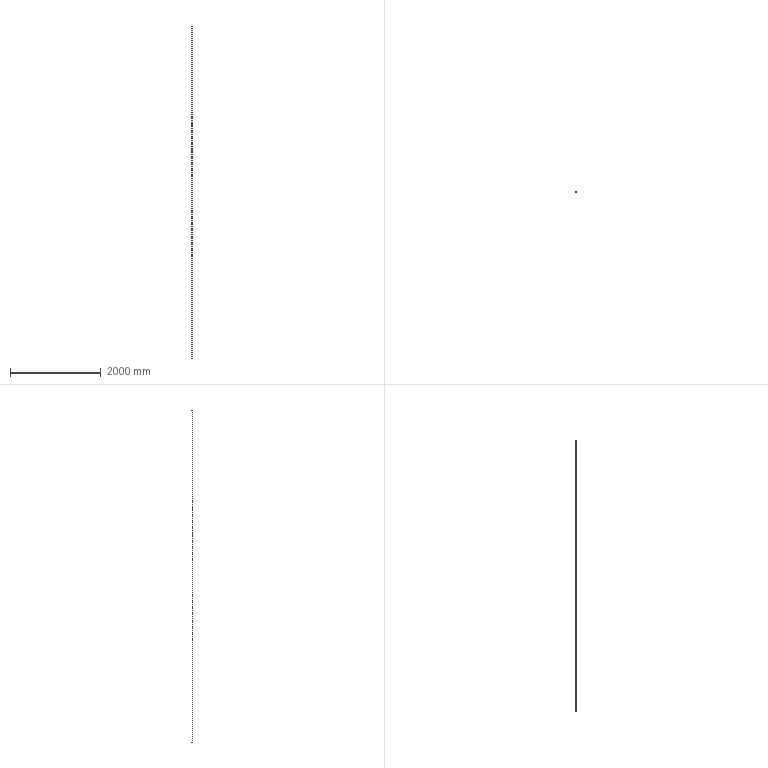Part | SolidWorks | features Extrusion 1 | 1 solid | 6 faces | box 19.05 x 19.05 x 7329 mm | volume 1032084 mm3 | cylinder 4 | plane 2 | commonest cylinder face diameters 13.55 x2 19.05 x2
STEP:
#1=CARTESIAN_POINT('',(-6.775,0.,3664.5));
#2=VERTEX_POINT('',#1);
#3=CARTESIAN_POINT('',(6.775,0.,3664.5));
#4=VERTEX_POINT('',#3);
#5=CARTESIAN_POINT('',(0.,0.,3664.5));
#6=DIRECTION('',(0.,0.,1.));
#7=DIRECTION('',(1.,0.,0.));
#8=AXIS2_PLACEMENT_3D('',#5,#6,#7);
#9=CIRCLE('',#8,6.775);
#10=EDGE_CURVE('',#2,#4,#9,.T.);
#11=ORIENTED_EDGE('',*,*,#10,.T.);
#12=CARTESIAN_POINT('',(6.775,0.,-3664.5));
#13=VERTEX_POINT('',#12);
#14=CARTESIAN_POINT('',(6.775,0.,3664.5));
#15=DIRECTION('',(0.,0.,-1.));
#16=VECTOR('',#15,1000.);
#17=LINE('',#14,#16);
#18=EDGE_CURVE('',#4,#13,#17,.T.);
#19=ORIENTED_EDGE('',*,*,#18,.T.);
#20=CARTESIAN_POINT('',(-6.775,0.,-3664.5));
#21=VERTEX_POINT('',#20);
#22=CARTESIAN_POINT('',(0.,0.,-3664.5));
#23=DIRECTION('',(0.,0.,1.));
#24=DIRECTION('',(1.,0.,0.));
#25=AXIS2_PLACEMENT_3D('',#22,#23,#24);
#26=CIRCLE('',#25,6.775);
#27=EDGE_CURVE('',#21,#13,#26,.T.);
#28=ORIENTED_EDGE('',*,*,#27,.F.);
#29=CARTESIAN_POINT('',(-6.775,0.,3664.5));
#30=DIRECTION('',(0.,0.,-1.));
#31=VECTOR('',#30,1000.);
#32=LINE('',#29,#31);
#33=EDGE_CURVE('',#2,#21,#32,.T.);
#34=ORIENTED_EDGE('',*,*,#33,.F.);
#35=EDGE_LOOP('',(#11,#19,#28,#34));
#36=FACE_OUTER_BOUND('',#35,.T.);
#37=CARTESIAN_POINT('',(0.,0.,3664.5));
#38=DIRECTION('',(0.,0.,-1.));
#39=DIRECTION('',(-1.,0.,0.));
#40=AXIS2_PLACEMENT_3D('',#37,#38,#39);
#41=CYLINDRICAL_SURFACE('',#40,6.775);
#42=ADVANCED_FACE('',(#36),#41,.F.);
#43=CARTESIAN_POINT('',(9.525,0.,3664.5));
#44=VERTEX_POINT('',#43);
#45=CARTESIAN_POINT('',(-9.525,0.,3664.5));
#46=VERTEX_POINT('',#45);
#47=CARTESIAN_POINT('',(0.,0.,3664.5));
#48=DIRECTION('',(0.,0.,1.));
#49=DIRECTION('',(1.,0.,0.));
#50=AXIS2_PLACEMENT_3D('',#47,#48,#49);
#51=CIRCLE('',#50,9.525);
#52=EDGE_CURVE('',#44,#46,#51,.T.);
#53=ORIENTED_EDGE('',*,*,#52,.F.);
#54=CARTESIAN_POINT('',(9.525,0.,-3664.5));
#55=VERTEX_POINT('',#54);
#56=CARTESIAN_POINT('',(9.525,0.,3664.5));
#57=DIRECTION('',(0.,0.,-1.));
#58=VECTOR('',#57,1000.);
#59=LINE('',#56,#58);
#60=EDGE_CURVE('',#44,#55,#59,.T.);
#61=ORIENTED_EDGE('',*,*,#60,.T.);
#62=CARTESIAN_POINT('',(-9.525,0.,-3664.5));
#63=VERTEX_POINT('',#62);
#64=CARTESIAN_POINT('',(0.,0.,-3664.5));
#65=DIRECTION('',(0.,0.,1.));
#66=DIRECTION('',(1.,0.,0.));
#67=AXIS2_PLACEMENT_3D('',#64,#65,#66);
#68=CIRCLE('',#67,9.525);
#69=EDGE_CURVE('',#55,#63,#68,.T.);
#70=ORIENTED_EDGE('',*,*,#69,.T.);
#71=CARTESIAN_POINT('',(-9.525,0.,3664.5));
#72=DIRECTION('',(0.,0.,-1.));
#73=VECTOR('',#72,1000.);
#74=LINE('',#71,#73);
#75=EDGE_CURVE('',#46,#63,#74,.T.);
#76=ORIENTED_EDGE('',*,*,#75,.F.);
#77=EDGE_LOOP('',(#53,#61,#70,#76));
#78=FACE_OUTER_BOUND('',#77,.T.);
#79=CARTESIAN_POINT('',(0.,0.,3664.5));
#80=DIRECTION('',(0.,0.,-1.));
#81=DIRECTION('',(-1.,0.,0.));
#82=AXIS2_PLACEMENT_3D('',#79,#80,#81);
#83=CYLINDRICAL_SURFACE('',#82,9.525);
#84=ADVANCED_FACE('',(#78),#83,.T.);
#85=CARTESIAN_POINT('',(0.,0.,3664.5));
#86=DIRECTION('',(0.,0.,1.));
#87=DIRECTION('',(1.,0.,0.));
#88=AXIS2_PLACEMENT_3D('',#85,#86,#87);
#89=CIRCLE('',#88,9.525);
#90=EDGE_CURVE('',#46,#44,#89,.T.);
#91=ORIENTED_EDGE('',*,*,#90,.T.);
#92=ORIENTED_EDGE('',*,*,#52,.T.);
#93=EDGE_LOOP('',(#91,#92));
#94=FACE_OUTER_BOUND('',#93,.T.);
#95=ORIENTED_EDGE('',*,*,#10,.F.);
#96=CARTESIAN_POINT('',(0.,0.,3664.5));
#97=DIRECTION('',(0.,0.,1.));
#98=DIRECTION('',(1.,0.,0.));
#99=AXIS2_PLACEMENT_3D('',#96,#97,#98);
#100=CIRCLE('',#99,6.775);
#101=EDGE_CURVE('',#4,#2,#100,.T.);
#102=ORIENTED_EDGE('',*,*,#101,.F.);
#103=EDGE_LOOP('',(#95,#102));
#104=FACE_BOUND('',#103,.T.);
#105=CARTESIAN_POINT('',(0.,0.,3664.5));
#106=DIRECTION('',(0.,0.,1.));
#107=DIRECTION('',(1.,0.,0.));
#108=AXIS2_PLACEMENT_3D('',#105,#106,#107);
#109=PLANE('',#108);
#110=ADVANCED_FACE('',(#94,#104),#109,.T.);
#111=CARTESIAN_POINT('',(0.,0.,-3664.5));
#112=DIRECTION('',(0.,0.,1.));
#113=DIRECTION('',(1.,0.,0.));
#114=AXIS2_PLACEMENT_3D('',#111,#112,#113);
#115=CIRCLE('',#114,9.525);
#116=EDGE_CURVE('',#63,#55,#115,.T.);
#117=ORIENTED_EDGE('',*,*,#116,.F.);
#118=ORIENTED_EDGE('',*,*,#69,.F.);
#119=EDGE_LOOP('',(#117,#118));
#120=FACE_OUTER_BOUND('',#119,.T.);
#121=ORIENTED_EDGE('',*,*,#27,.T.);
#122=CARTESIAN_POINT('',(0.,0.,-3664.5));
#123=DIRECTION('',(0.,0.,1.));
#124=DIRECTION('',(1.,0.,0.));
#125=AXIS2_PLACEMENT_3D('',#122,#123,#124);
#126=CIRCLE('',#125,6.775);
#127=EDGE_CURVE('',#13,#21,#126,.T.);
#128=ORIENTED_EDGE('',*,*,#127,.T.);
#129=EDGE_LOOP('',(#121,#128));
#130=FACE_BOUND('',#129,.T.);
#131=CARTESIAN_POINT('',(0.,0.,-3664.5));
#132=DIRECTION('',(0.,0.,1.));
#133=DIRECTION('',(1.,0.,0.));
#134=AXIS2_PLACEMENT_3D('',#131,#132,#133);
#135=PLANE('',#134);
#136=ADVANCED_FACE('',(#120,#130),#135,.F.);
#137=ORIENTED_EDGE('',*,*,#60,.F.);
#138=ORIENTED_EDGE('',*,*,#90,.F.);
#139=ORIENTED_EDGE('',*,*,#75,.T.);
#140=ORIENTED_EDGE('',*,*,#116,.T.);
#141=EDGE_LOOP('',(#137,#138,#139,#140));
#142=FACE_OUTER_BOUND('',#141,.T.);
#143=CARTESIAN_POINT('',(0.,0.,3664.5));
#144=DIRECTION('',(0.,0.,-1.));
#145=DIRECTION('',(-1.,0.,0.));
#146=AXIS2_PLACEMENT_3D('',#143,#144,#145);
#147=CYLINDRICAL_SURFACE('',#146,9.525);
#148=ADVANCED_FACE('',(#142),#147,.T.);
#149=ORIENTED_EDGE('',*,*,#18,.F.);
#150=ORIENTED_EDGE('',*,*,#101,.T.);
#151=ORIENTED_EDGE('',*,*,#33,.T.);
#152=ORIENTED_EDGE('',*,*,#127,.F.);
#153=EDGE_LOOP('',(#149,#150,#151,#152));
#154=FACE_OUTER_BOUND('',#153,.T.);
#155=CARTESIAN_POINT('',(0.,0.,3664.5));
#156=DIRECTION('',(0.,0.,-1.));
#157=DIRECTION('',(-1.,0.,0.));
#158=AXIS2_PLACEMENT_3D('',#155,#156,#157);
#159=CYLINDRICAL_SURFACE('',#158,6.775);
#160=ADVANCED_FACE('',(#154),#159,.F.);
#161=CLOSED_SHELL('',(#42,#84,#110,#136,#148,#160));
#162=MANIFOLD_SOLID_BREP('',#161);
#163=CARTESIAN_POINT('',(0.,0.,0.));
#164=DIRECTION('',(0.,0.,1.));
#165=DIRECTION('',(1.,0.,0.));
#166=AXIS2_PLACEMENT_3D('',#163,#164,#165);
#167=(LENGTH_UNIT()NAMED_UNIT(*)SI_UNIT(.MILLI.,.METRE.));
#168=UNCERTAINTY_MEASURE_WITH_UNIT(LENGTH_MEASURE(0.00001),#167,'','');
#169=(NAMED_UNIT(*)PLANE_ANGLE_UNIT()SI_UNIT($,.RADIAN.));
#170=(NAMED_UNIT(*)SI_UNIT($,.STERADIAN.)SOLID_ANGLE_UNIT());
#171=(GEOMETRIC_REPRESENTATION_CONTEXT(3)GLOBAL_UNCERTAINTY_ASSIGNED_CONTEXT((#168))GLOBAL_UNIT_ASSIGNED_CONTEXT((#167,#169,#170))REPRESENTATION_CONTEXT('',''));
#172=ADVANCED_BREP_SHAPE_REPRESENTATION('',(#162,#166),#171);